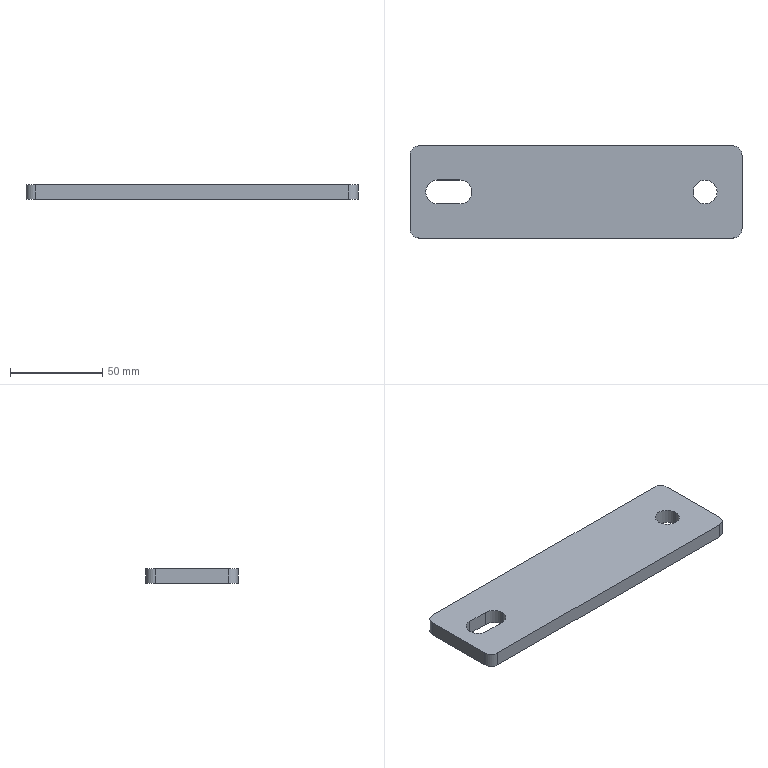Part | STEP file | IN-01-01-03-02 | 1 solid | 17 faces | box 180 x 50 x 8 mm | volume 68457 mm3 | cylinder 9 | plane 8 | commonest cylinder face diameters 13 x5 10 x4
STEP:
#1=CARTESIAN_POINT('',(0.,0.,0.));
#2=DIRECTION('',(0.,0.,1.));
#3=DIRECTION('',(1.,0.,0.));
#4=AXIS2_PLACEMENT_3D('',#1,#2,#3);
#5=CARTESIAN_POINT('',(27.,-18.5,8.));
#6=VERTEX_POINT('',#5);
#7=CARTESIAN_POINT('',(27.,-18.5,0.));
#8=VERTEX_POINT('',#7);
#9=CARTESIAN_POINT('',(27.,-18.5,0.));
#10=DIRECTION('',(0.,0.,-1.));
#11=VECTOR('',#10,1.);
#12=LINE('',#9,#11);
#13=CARTESIAN_POINT('',(27.,-25.,0.));
#14=DIRECTION('',(0.,0.,1.));
#15=DIRECTION('',(1.,0.,0.));
#16=AXIS2_PLACEMENT_3D('',#13,#14,#15);
#17=CYLINDRICAL_SURFACE('',#16,6.5);
#18=CARTESIAN_POINT('',(1.571,0.));
#19=DIRECTION('',(0.,-1.));
#20=VECTOR('',#19,1.);
#21=LINE('',#18,#20);
#22=(GEOMETRIC_REPRESENTATION_CONTEXT(2)PARAMETRIC_REPRESENTATION_CONTEXT()REPRESENTATION_CONTEXT('',''));
#23=DEFINITIONAL_REPRESENTATION('',(#21),#22);
#24=PCURVE('',#17,#23);
#25=CARTESIAN_POINT('',(27.,-18.5,0.));
#26=DIRECTION('',(0.,1.,0.));
#27=DIRECTION('',(0.,0.,1.));
#28=AXIS2_PLACEMENT_3D('',#25,#26,#27);
#29=PLANE('',#28);
#30=CARTESIAN_POINT('',(0.,0.));
#31=DIRECTION('',(-1.,0.));
#32=VECTOR('',#31,1.);
#33=LINE('',#30,#32);
#34=(GEOMETRIC_REPRESENTATION_CONTEXT(2)PARAMETRIC_REPRESENTATION_CONTEXT()REPRESENTATION_CONTEXT('',''));
#35=DEFINITIONAL_REPRESENTATION('',(#33),#34);
#36=PCURVE('',#29,#35);
#37=SURFACE_CURVE('',#12,(#24,#36),.PCURVE_S1.);
#38=EDGE_CURVE('',#6,#8,#37,.T.);
#39=ORIENTED_EDGE('',*,*,#38,.F.);
#40=CARTESIAN_POINT('',(33.5,-25.,8.));
#41=VERTEX_POINT('',#40);
#42=CARTESIAN_POINT('',(27.,-25.,8.));
#43=DIRECTION('',(0.,0.,-1.));
#44=DIRECTION('',(1.,0.,0.));
#45=AXIS2_PLACEMENT_3D('',#42,#43,#44);
#46=CIRCLE('',#45,6.5);
#47=CARTESIAN_POINT('',(6.283,8.));
#48=DIRECTION('',(-1.,0.));
#49=VECTOR('',#48,1.);
#50=LINE('',#47,#49);
#51=(GEOMETRIC_REPRESENTATION_CONTEXT(2)PARAMETRIC_REPRESENTATION_CONTEXT()REPRESENTATION_CONTEXT('',''));
#52=DEFINITIONAL_REPRESENTATION('',(#50),#51);
#53=PCURVE('',#17,#52);
#54=CARTESIAN_POINT('',(90.,-25.,8.));
#55=DIRECTION('',(0.,0.,1.));
#56=DIRECTION('',(1.,0.,0.));
#57=AXIS2_PLACEMENT_3D('',#54,#55,#56);
#58=PLANE('',#57);
#59=CARTESIAN_POINT('',(-56.5,0.));
#60=CARTESIAN_POINT('',(-56.5,-11.258));
#61=CARTESIAN_POINT('',(-66.25,-5.629));
#62=CARTESIAN_POINT('',(-76.,0.));
#63=CARTESIAN_POINT('',(-66.25,5.629));
#64=CARTESIAN_POINT('',(-56.5,11.258));
#65=CARTESIAN_POINT('',(-56.5,0.));
#66=(BOUNDED_CURVE()B_SPLINE_CURVE(2,(#59,#60,#61,#62,#63,#64,#65),.UNSPECIFIED.,.T.,.F.)B_SPLINE_CURVE_WITH_KNOTS((1,2,2,2,2,1),(-2.094,0.,2.094,4.189,6.283,8.378),.UNSPECIFIED.)CURVE()GEOMETRIC_REPRESENTATION_ITEM()RATIONAL_B_SPLINE_CURVE((1.,0.5,1.,0.5,1.,0.5,1.))REPRESENTATION_ITEM(''));
#67=(GEOMETRIC_REPRESENTATION_CONTEXT(2)PARAMETRIC_REPRESENTATION_CONTEXT()REPRESENTATION_CONTEXT('',''));
#68=DEFINITIONAL_REPRESENTATION('',(#66),#67);
#69=PCURVE('',#58,#68);
#70=SURFACE_CURVE('',#46,(#53,#69),.PCURVE_S1.);
#71=EDGE_CURVE('',#6,#41,#70,.T.);
#72=ORIENTED_EDGE('',*,*,#71,.T.);
#73=CARTESIAN_POINT('',(33.5,-25.,0.));
#74=VERTEX_POINT('',#73);
#75=CARTESIAN_POINT('',(33.5,-25.,0.));
#76=DIRECTION('',(0.,0.,1.));
#77=VECTOR('',#76,1.);
#78=LINE('',#75,#77);
#79=CARTESIAN_POINT('',(0.,0.));
#80=DIRECTION('',(0.,1.));
#81=VECTOR('',#80,1.);
#82=LINE('',#79,#81);
#83=(GEOMETRIC_REPRESENTATION_CONTEXT(2)PARAMETRIC_REPRESENTATION_CONTEXT()REPRESENTATION_CONTEXT('',''));
#84=DEFINITIONAL_REPRESENTATION('',(#82),#83);
#85=PCURVE('',#17,#84);
#86=CARTESIAN_POINT('',(27.,-25.,0.));
#87=DIRECTION('',(0.,0.,1.));
#88=DIRECTION('',(1.,0.,0.));
#89=AXIS2_PLACEMENT_3D('',#86,#87,#88);
#90=CYLINDRICAL_SURFACE('',#89,6.5);
#91=CARTESIAN_POINT('',(6.283,0.));
#92=DIRECTION('',(0.,1.));
#93=VECTOR('',#92,1.);
#94=LINE('',#91,#93);
#95=(GEOMETRIC_REPRESENTATION_CONTEXT(2)PARAMETRIC_REPRESENTATION_CONTEXT()REPRESENTATION_CONTEXT('',''));
#96=DEFINITIONAL_REPRESENTATION('',(#94),#95);
#97=PCURVE('',#90,#96);
#98=SURFACE_CURVE('',#78,(#85,#97),.PCURVE_S1.);
#99=EDGE_CURVE('',#74,#41,#98,.T.);
#100=ORIENTED_EDGE('',*,*,#99,.F.);
#101=CARTESIAN_POINT('',(27.,-25.,0.));
#102=DIRECTION('',(0.,0.,-1.));
#103=DIRECTION('',(1.,0.,0.));
#104=AXIS2_PLACEMENT_3D('',#101,#102,#103);
#105=CIRCLE('',#104,6.5);
#106=CARTESIAN_POINT('',(6.283,0.));
#107=DIRECTION('',(-1.,0.));
#108=VECTOR('',#107,1.);
#109=LINE('',#106,#108);
#110=(GEOMETRIC_REPRESENTATION_CONTEXT(2)PARAMETRIC_REPRESENTATION_CONTEXT()REPRESENTATION_CONTEXT('',''));
#111=DEFINITIONAL_REPRESENTATION('',(#109),#110);
#112=PCURVE('',#17,#111);
#113=CARTESIAN_POINT('',(90.,-25.,0.));
#114=DIRECTION('',(0.,0.,1.));
#115=DIRECTION('',(1.,0.,0.));
#116=AXIS2_PLACEMENT_3D('',#113,#114,#115);
#117=PLANE('',#116);
#118=CARTESIAN_POINT('',(-56.5,0.));
#119=CARTESIAN_POINT('',(-56.5,-11.258));
#120=CARTESIAN_POINT('',(-66.25,-5.629));
#121=CARTESIAN_POINT('',(-76.,0.));
#122=CARTESIAN_POINT('',(-66.25,5.629));
#123=CARTESIAN_POINT('',(-56.5,11.258));
#124=CARTESIAN_POINT('',(-56.5,0.));
#125=(BOUNDED_CURVE()B_SPLINE_CURVE(2,(#118,#119,#120,#121,#122,#123,#124),.UNSPECIFIED.,.T.,.F.)B_SPLINE_CURVE_WITH_KNOTS((1,2,2,2,2,1),(-2.094,0.,2.094,4.189,6.283,8.378),.UNSPECIFIED.)CURVE()GEOMETRIC_REPRESENTATION_ITEM()RATIONAL_B_SPLINE_CURVE((1.,0.5,1.,0.5,1.,0.5,1.))REPRESENTATION_ITEM(''));
#126=(GEOMETRIC_REPRESENTATION_CONTEXT(2)PARAMETRIC_REPRESENTATION_CONTEXT()REPRESENTATION_CONTEXT('',''));
#127=DEFINITIONAL_REPRESENTATION('',(#125),#126);
#128=PCURVE('',#117,#127);
#129=SURFACE_CURVE('',#105,(#112,#128),.PCURVE_S1.);
#130=EDGE_CURVE('',#8,#74,#129,.T.);
#131=ORIENTED_EDGE('',*,*,#130,.F.);
#132=EDGE_LOOP('',(#39,#72,#100,#131));
#133=FACE_BOUND('',#132,.F.);
#134=ADVANCED_FACE('',(#133),#17,.F.);
#135=CARTESIAN_POINT('',(166.5,-25.,0.));
#136=VERTEX_POINT('',#135);
#137=CARTESIAN_POINT('',(166.5,-25.,8.));
#138=VERTEX_POINT('',#137);
#139=CARTESIAN_POINT('',(166.5,-25.,0.));
#140=DIRECTION('',(0.,0.,1.));
#141=VECTOR('',#140,1.);
#142=LINE('',#139,#141);
#143=CARTESIAN_POINT('',(160.,-25.,0.));
#144=DIRECTION('',(0.,0.,1.));
#145=DIRECTION('',(1.,0.,0.));
#146=AXIS2_PLACEMENT_3D('',#143,#144,#145);
#147=CYLINDRICAL_SURFACE('',#146,6.5);
#148=CARTESIAN_POINT('',(6.283,0.));
#149=DIRECTION('',(0.,1.));
#150=VECTOR('',#149,1.);
#151=LINE('',#148,#150);
#152=(GEOMETRIC_REPRESENTATION_CONTEXT(2)PARAMETRIC_REPRESENTATION_CONTEXT()REPRESENTATION_CONTEXT('',''));
#153=DEFINITIONAL_REPRESENTATION('',(#151),#152);
#154=PCURVE('',#147,#153);
#155=CARTESIAN_POINT('',(160.,-25.,0.));
#156=DIRECTION('',(0.,0.,1.));
#157=DIRECTION('',(1.,0.,0.));
#158=AXIS2_PLACEMENT_3D('',#155,#156,#157);
#159=CYLINDRICAL_SURFACE('',#158,6.5);
#160=CARTESIAN_POINT('',(0.,0.));
#161=DIRECTION('',(0.,1.));
#162=VECTOR('',#161,1.);
#163=LINE('',#160,#162);
#164=(GEOMETRIC_REPRESENTATION_CONTEXT(2)PARAMETRIC_REPRESENTATION_CONTEXT()REPRESENTATION_CONTEXT('',''));
#165=DEFINITIONAL_REPRESENTATION('',(#163),#164);
#166=PCURVE('',#159,#165);
#167=SURFACE_CURVE('',#142,(#154,#166),.PCURVE_S1.);
#168=EDGE_CURVE('',#136,#138,#167,.T.);
#169=ORIENTED_EDGE('',*,*,#168,.T.);
#170=CARTESIAN_POINT('',(153.5,-25.,8.));
#171=VERTEX_POINT('',#170);
#172=CARTESIAN_POINT('',(160.,-25.,8.));
#173=DIRECTION('',(0.,0.,-1.));
#174=DIRECTION('',(1.,0.,0.));
#175=AXIS2_PLACEMENT_3D('',#172,#173,#174);
#176=CIRCLE('',#175,6.5);
#177=CARTESIAN_POINT('',(6.283,8.));
#178=DIRECTION('',(-1.,0.));
#179=VECTOR('',#178,1.);
#180=LINE('',#177,#179);
#181=(GEOMETRIC_REPRESENTATION_CONTEXT(2)PARAMETRIC_REPRESENTATION_CONTEXT()REPRESENTATION_CONTEXT('',''));
#182=DEFINITIONAL_REPRESENTATION('',(#180),#181);
#183=PCURVE('',#147,#182);
#184=CARTESIAN_POINT('',(76.5,0.));
#185=CARTESIAN_POINT('',(76.5,-11.258));
#186=CARTESIAN_POINT('',(66.75,-5.629));
#187=CARTESIAN_POINT('',(57.,0.));
#188=CARTESIAN_POINT('',(66.75,5.629));
#189=CARTESIAN_POINT('',(76.5,11.258));
#190=CARTESIAN_POINT('',(76.5,0.));
#191=(BOUNDED_CURVE()B_SPLINE_CURVE(2,(#184,#185,#186,#187,#188,#189,#190),.UNSPECIFIED.,.T.,.F.)B_SPLINE_CURVE_WITH_KNOTS((1,2,2,2,2,1),(-2.094,0.,2.094,4.189,6.283,8.378),.UNSPECIFIED.)CURVE()GEOMETRIC_REPRESENTATION_ITEM()RATIONAL_B_SPLINE_CURVE((1.,0.5,1.,0.5,1.,0.5,1.))REPRESENTATION_ITEM(''));
#192=(GEOMETRIC_REPRESENTATION_CONTEXT(2)PARAMETRIC_REPRESENTATION_CONTEXT()REPRESENTATION_CONTEXT('',''));
#193=DEFINITIONAL_REPRESENTATION('',(#191),#192);
#194=PCURVE('',#58,#193);
#195=SURFACE_CURVE('',#176,(#183,#194),.PCURVE_S1.);
#196=EDGE_CURVE('',#138,#171,#195,.T.);
#197=ORIENTED_EDGE('',*,*,#196,.T.);
#198=CARTESIAN_POINT('',(153.5,-25.,0.));
#199=VERTEX_POINT('',#198);
#200=CARTESIAN_POINT('',(153.5,-25.,0.));
#201=DIRECTION('',(0.,0.,1.));
#202=VECTOR('',#201,1.);
#203=LINE('',#200,#202);
#204=CARTESIAN_POINT('',(3.142,0.));
#205=DIRECTION('',(0.,1.));
#206=VECTOR('',#205,1.);
#207=LINE('',#204,#206);
#208=(GEOMETRIC_REPRESENTATION_CONTEXT(2)PARAMETRIC_REPRESENTATION_CONTEXT()REPRESENTATION_CONTEXT('',''));
#209=DEFINITIONAL_REPRESENTATION('',(#207),#208);
#210=PCURVE('',#147,#209);
#211=CARTESIAN_POINT('',(3.142,0.));
#212=DIRECTION('',(0.,1.));
#213=VECTOR('',#212,1.);
#214=LINE('',#211,#213);
#215=(GEOMETRIC_REPRESENTATION_CONTEXT(2)PARAMETRIC_REPRESENTATION_CONTEXT()REPRESENTATION_CONTEXT('',''));
#216=DEFINITIONAL_REPRESENTATION('',(#214),#215);
#217=PCURVE('',#159,#216);
#218=SURFACE_CURVE('',#203,(#210,#217),.PCURVE_S1.);
#219=EDGE_CURVE('',#199,#171,#218,.T.);
#220=ORIENTED_EDGE('',*,*,#219,.F.);
#221=CARTESIAN_POINT('',(160.,-25.,0.));
#222=DIRECTION('',(0.,0.,-1.));
#223=DIRECTION('',(1.,0.,0.));
#224=AXIS2_PLACEMENT_3D('',#221,#222,#223);
#225=CIRCLE('',#224,6.5);
#226=CARTESIAN_POINT('',(6.283,0.));
#227=DIRECTION('',(-1.,0.));
#228=VECTOR('',#227,1.);
#229=LINE('',#226,#228);
#230=(GEOMETRIC_REPRESENTATION_CONTEXT(2)PARAMETRIC_REPRESENTATION_CONTEXT()REPRESENTATION_CONTEXT('',''));
#231=DEFINITIONAL_REPRESENTATION('',(#229),#230);
#232=PCURVE('',#147,#231);
#233=CARTESIAN_POINT('',(76.5,0.));
#234=CARTESIAN_POINT('',(76.5,-11.258));
#235=CARTESIAN_POINT('',(66.75,-5.629));
#236=CARTESIAN_POINT('',(57.,0.));
#237=CARTESIAN_POINT('',(66.75,5.629));
#238=CARTESIAN_POINT('',(76.5,11.258));
#239=CARTESIAN_POINT('',(76.5,0.));
#240=(BOUNDED_CURVE()B_SPLINE_CURVE(2,(#233,#234,#235,#236,#237,#238,#239),.UNSPECIFIED.,.T.,.F.)B_SPLINE_CURVE_WITH_KNOTS((1,2,2,2,2,1),(-2.094,0.,2.094,4.189,6.283,8.378),.UNSPECIFIED.)CURVE()GEOMETRIC_REPRESENTATION_ITEM()RATIONAL_B_SPLINE_CURVE((1.,0.5,1.,0.5,1.,0.5,1.))REPRESENTATION_ITEM(''));
#241=(GEOMETRIC_REPRESENTATION_CONTEXT(2)PARAMETRIC_REPRESENTATION_CONTEXT()REPRESENTATION_CONTEXT('',''));
#242=DEFINITIONAL_REPRESENTATION('',(#240),#241);
#243=PCURVE('',#117,#242);
#244=SURFACE_CURVE('',#225,(#232,#243),.PCURVE_S1.);
#245=EDGE_CURVE('',#136,#199,#244,.T.);
#246=ORIENTED_EDGE('',*,*,#245,.F.);
#247=EDGE_LOOP('',(#169,#197,#220,#246));
#248=FACE_BOUND('',#247,.F.);
#249=ADVANCED_FACE('',(#248),#147,.F.);
#250=CARTESIAN_POINT('',(15.,-31.5,0.));
#251=VERTEX_POINT('',#250);
#252=CARTESIAN_POINT('',(15.,-18.5,0.));
#253=VERTEX_POINT('',#252);
#254=CARTESIAN_POINT('',(15.,-25.,0.));
#255=DIRECTION('',(0.,0.,-1.));
#256=DIRECTION('',(1.,0.,0.));
#257=AXIS2_PLACEMENT_3D('',#254,#255,#256);
#258=CIRCLE('',#257,6.5);
#259=CARTESIAN_POINT('',(-68.5,0.));
#260=CARTESIAN_POINT('',(-68.5,-11.258));
#261=CARTESIAN_POINT('',(-78.25,-5.629));
#262=CARTESIAN_POINT('',(-88.,0.));
#263=CARTESIAN_POINT('',(-78.25,5.629));
#264=CARTESIAN_POINT('',(-68.5,11.258));
#265=CARTESIAN_POINT('',(-68.5,0.));
#266=(BOUNDED_CURVE()B_SPLINE_CURVE(2,(#259,#260,#261,#262,#263,#264,#265),.UNSPECIFIED.,.T.,.F.)B_SPLINE_CURVE_WITH_KNOTS((1,2,2,2,2,1),(-2.094,0.,2.094,4.189,6.283,8.378),.UNSPECIFIED.)CURVE()GEOMETRIC_REPRESENTATION_ITEM()RATIONAL_B_SPLINE_CURVE((1.,0.5,1.,0.5,1.,0.5,1.))REPRESENTATION_ITEM(''));
#267=(GEOMETRIC_REPRESENTATION_CONTEXT(2)PARAMETRIC_REPRESENTATION_CONTEXT()REPRESENTATION_CONTEXT('',''));
#268=DEFINITIONAL_REPRESENTATION('',(#266),#267);
#269=PCURVE('',#117,#268);
#270=CARTESIAN_POINT('',(15.,-25.,0.));
#271=DIRECTION('',(0.,0.,1.));
#272=DIRECTION('',(1.,0.,0.));
#273=AXIS2_PLACEMENT_3D('',#270,#271,#272);
#274=CYLINDRICAL_SURFACE('',#273,6.5);
#275=CARTESIAN_POINT('',(6.283,0.));
#276=DIRECTION('',(-1.,0.));
#277=VECTOR('',#276,1.);
#278=LINE('',#275,#277);
#279=(GEOMETRIC_REPRESENTATION_CONTEXT(2)PARAMETRIC_REPRESENTATION_CONTEXT()REPRESENTATION_CONTEXT('',''));
#280=DEFINITIONAL_REPRESENTATION('',(#278),#279);
#281=PCURVE('',#274,#280);
#282=SURFACE_CURVE('',#258,(#269,#281),.PCURVE_S1.);
#283=EDGE_CURVE('',#251,#253,#282,.T.);
#284=ORIENTED_EDGE('',*,*,#283,.F.);
#285=CARTESIAN_POINT('',(27.,-31.5,0.));
#286=VERTEX_POINT('',#285);
#287=CARTESIAN_POINT('',(90.,-31.5,0.));
#288=DIRECTION('',(-1.,0.,0.));
#289=VECTOR('',#288,1.);
#290=LINE('',#287,#289);
#291=CARTESIAN_POINT('',(0.,-6.5));
#292=DIRECTION('',(-1.,0.));
#293=VECTOR('',#292,1.);
#294=LINE('',#291,#293);
#295=(GEOMETRIC_REPRESENTATION_CONTEXT(2)PARAMETRIC_REPRESENTATION_CONTEXT()REPRESENTATION_CONTEXT('',''));
#296=DEFINITIONAL_REPRESENTATION('',(#294),#295);
#297=PCURVE('',#117,#296);
#298=CARTESIAN_POINT('',(15.,-31.5,0.));
#299=DIRECTION('',(0.,-1.,0.));
#300=DIRECTION('',(0.,0.,-1.));
#301=AXIS2_PLACEMENT_3D('',#298,#299,#300);
#302=PLANE('',#301);
#303=CARTESIAN_POINT('',(0.,75.));
#304=DIRECTION('',(0.,-1.));
#305=VECTOR('',#304,1.);
#306=LINE('',#303,#305);
#307=(GEOMETRIC_REPRESENTATION_CONTEXT(2)PARAMETRIC_REPRESENTATION_CONTEXT()REPRESENTATION_CONTEXT('',''));
#308=DEFINITIONAL_REPRESENTATION('',(#306),#307);
#309=PCURVE('',#302,#308);
#310=SURFACE_CURVE('',#290,(#297,#309),.PCURVE_S1.);
#311=EDGE_CURVE('',#286,#251,#310,.T.);
#312=ORIENTED_EDGE('',*,*,#311,.F.);
#313=CARTESIAN_POINT('',(27.,-25.,0.));
#314=DIRECTION('',(0.,0.,-1.));
#315=DIRECTION('',(1.,0.,0.));
#316=AXIS2_PLACEMENT_3D('',#313,#314,#315);
#317=CIRCLE('',#316,6.5);
#318=CARTESIAN_POINT('',(-56.5,0.));
#319=CARTESIAN_POINT('',(-56.5,-11.258));
#320=CARTESIAN_POINT('',(-66.25,-5.629));
#321=CARTESIAN_POINT('',(-76.,0.));
#322=CARTESIAN_POINT('',(-66.25,5.629));
#323=CARTESIAN_POINT('',(-56.5,11.258));
#324=CARTESIAN_POINT('',(-56.5,0.));
#325=(BOUNDED_CURVE()B_SPLINE_CURVE(2,(#318,#319,#320,#321,#322,#323,#324),.UNSPECIFIED.,.T.,.F.)B_SPLINE_CURVE_WITH_KNOTS((1,2,2,2,2,1),(-2.094,0.,2.094,4.189,6.283,8.378),.UNSPECIFIED.)CURVE()GEOMETRIC_REPRESENTATION_ITEM()RATIONAL_B_SPLINE_CURVE((1.,0.5,1.,0.5,1.,0.5,1.))REPRESENTATION_ITEM(''));
#326=(GEOMETRIC_REPRESENTATION_CONTEXT(2)PARAMETRIC_REPRESENTATION_CONTEXT()REPRESENTATION_CONTEXT('',''));
#327=DEFINITIONAL_REPRESENTATION('',(#325),#326);
#328=PCURVE('',#117,#327);
#329=CARTESIAN_POINT('',(6.283,0.));
#330=DIRECTION('',(-1.,0.));
#331=VECTOR('',#330,1.);
#332=LINE('',#329,#331);
#333=(GEOMETRIC_REPRESENTATION_CONTEXT(2)PARAMETRIC_REPRESENTATION_CONTEXT()REPRESENTATION_CONTEXT('',''));
#334=DEFINITIONAL_REPRESENTATION('',(#332),#333);
#335=PCURVE('',#90,#334);
#336=SURFACE_CURVE('',#317,(#328,#335),.PCURVE_S1.);
#337=EDGE_CURVE('',#74,#286,#336,.T.);
#338=ORIENTED_EDGE('',*,*,#337,.F.);
#339=ORIENTED_EDGE('',*,*,#130,.F.);
#340=CARTESIAN_POINT('',(90.,-18.5,0.));
#341=DIRECTION('',(1.,0.,0.));
#342=VECTOR('',#341,1.);
#343=LINE('',#340,#342);
#344=CARTESIAN_POINT('',(0.,6.5));
#345=DIRECTION('',(1.,0.));
#346=VECTOR('',#345,1.);
#347=LINE('',#344,#346);
#348=(GEOMETRIC_REPRESENTATION_CONTEXT(2)PARAMETRIC_REPRESENTATION_CONTEXT()REPRESENTATION_CONTEXT('',''));
#349=DEFINITIONAL_REPRESENTATION('',(#347),#348);
#350=PCURVE('',#117,#349);
#351=CARTESIAN_POINT('',(0.,63.));
#352=DIRECTION('',(0.,1.));
#353=VECTOR('',#352,1.);
#354=LINE('',#351,#353);
#355=(GEOMETRIC_REPRESENTATION_CONTEXT(2)PARAMETRIC_REPRESENTATION_CONTEXT()REPRESENTATION_CONTEXT('',''));
#356=DEFINITIONAL_REPRESENTATION('',(#354),#355);
#357=PCURVE('',#29,#356);
#358=SURFACE_CURVE('',#343,(#350,#357),.PCURVE_S1.);
#359=EDGE_CURVE('',#253,#8,#358,.T.);
#360=ORIENTED_EDGE('',*,*,#359,.F.);
#361=EDGE_LOOP('',(#284,#312,#338,#339,#360));
#362=FACE_BOUND('',#361,.T.);
#363=ORIENTED_EDGE('',*,*,#245,.F.);
#364=CARTESIAN_POINT('',(160.,-25.,0.));
#365=DIRECTION('',(0.,0.,-1.));
#366=DIRECTION('',(1.,0.,0.));
#367=AXIS2_PLACEMENT_3D('',#364,#365,#366);
#368=CIRCLE('',#367,6.5);
#369=CARTESIAN_POINT('',(76.5,0.));
#370=CARTESIAN_POINT('',(76.5,-11.258));
#371=CARTESIAN_POINT('',(66.75,-5.629));
#372=CARTESIAN_POINT('',(57.,0.));
#373=CARTESIAN_POINT('',(66.75,5.629));
#374=CARTESIAN_POINT('',(76.5,11.258));
#375=CARTESIAN_POINT('',(76.5,0.));
#376=(BOUNDED_CURVE()B_SPLINE_CURVE(2,(#369,#370,#371,#372,#373,#374,#375),.UNSPECIFIED.,.T.,.F.)B_SPLINE_CURVE_WITH_KNOTS((1,2,2,2,2,1),(-2.094,0.,2.094,4.189,6.283,8.378),.UNSPECIFIED.)CURVE()GEOMETRIC_REPRESENTATION_ITEM()RATIONAL_B_SPLINE_CURVE((1.,0.5,1.,0.5,1.,0.5,1.))REPRESENTATION_ITEM(''));
#377=(GEOMETRIC_REPRESENTATION_CONTEXT(2)PARAMETRIC_REPRESENTATION_CONTEXT()REPRESENTATION_CONTEXT('',''));
#378=DEFINITIONAL_REPRESENTATION('',(#376),#377);
#379=PCURVE('',#117,#378);
#380=CARTESIAN_POINT('',(6.283,0.));
#381=DIRECTION('',(-1.,0.));
#382=VECTOR('',#381,1.);
#383=LINE('',#380,#382);
#384=(GEOMETRIC_REPRESENTATION_CONTEXT(2)PARAMETRIC_REPRESENTATION_CONTEXT()REPRESENTATION_CONTEXT('',''));
#385=DEFINITIONAL_REPRESENTATION('',(#383),#384);
#386=PCURVE('',#159,#385);
#387=SURFACE_CURVE('',#368,(#379,#386),.PCURVE_S1.);
#388=EDGE_CURVE('',#199,#136,#387,.T.);
#389=ORIENTED_EDGE('',*,*,#388,.F.);
#390=EDGE_LOOP('',(#363,#389));
#391=FACE_BOUND('',#390,.T.);
#392=CARTESIAN_POINT('',(5.,0.,0.));
#393=VERTEX_POINT('',#392);
#394=CARTESIAN_POINT('',(0.,-5.,0.));
#395=VERTEX_POINT('',#394);
#396=CARTESIAN_POINT('',(5.,-5.,0.));
#397=DIRECTION('',(0.,0.,1.));
#398=DIRECTION('',(1.,0.,0.));
#399=AXIS2_PLACEMENT_3D('',#396,#397,#398);
#400=CIRCLE('',#399,5.);
#401=CARTESIAN_POINT('',(-85.,20.));
#402=DIRECTION('',(1.,0.));
#403=AXIS2_PLACEMENT_2D('',#401,#402);
#404=CIRCLE('',#403,5.);
#405=(GEOMETRIC_REPRESENTATION_CONTEXT(2)PARAMETRIC_REPRESENTATION_CONTEXT()REPRESENTATION_CONTEXT('',''));
#406=DEFINITIONAL_REPRESENTATION('',(#404),#405);
#407=PCURVE('',#117,#406);
#408=CARTESIAN_POINT('',(5.,-5.,0.));
#409=DIRECTION('',(0.,0.,1.));
#410=DIRECTION('',(1.,0.,0.));
#411=AXIS2_PLACEMENT_3D('',#408,#409,#410);
#412=CYLINDRICAL_SURFACE('',#411,5.);
#413=CARTESIAN_POINT('',(0.,0.));
#414=DIRECTION('',(1.,0.));
#415=VECTOR('',#414,1.);
#416=LINE('',#413,#415);
#417=(GEOMETRIC_REPRESENTATION_CONTEXT(2)PARAMETRIC_REPRESENTATION_CONTEXT()REPRESENTATION_CONTEXT('',''));
#418=DEFINITIONAL_REPRESENTATION('',(#416),#417);
#419=PCURVE('',#412,#418);
#420=SURFACE_CURVE('',#400,(#407,#419),.PCURVE_S1.);
#421=EDGE_CURVE('',#393,#395,#420,.T.);
#422=ORIENTED_EDGE('',*,*,#421,.F.);
#423=CARTESIAN_POINT('',(175.,0.,0.));
#424=VERTEX_POINT('',#423);
#425=CARTESIAN_POINT('',(90.,0.,0.));
#426=DIRECTION('',(-1.,0.,0.));
#427=VECTOR('',#426,1.);
#428=LINE('',#425,#427);
#429=CARTESIAN_POINT('',(0.,25.));
#430=DIRECTION('',(-1.,0.));
#431=VECTOR('',#430,1.);
#432=LINE('',#429,#431);
#433=(GEOMETRIC_REPRESENTATION_CONTEXT(2)PARAMETRIC_REPRESENTATION_CONTEXT()REPRESENTATION_CONTEXT('',''));
#434=DEFINITIONAL_REPRESENTATION('',(#432),#433);
#435=PCURVE('',#117,#434);
#436=CARTESIAN_POINT('',(175.,0.,0.));
#437=DIRECTION('',(0.,1.,0.));
#438=DIRECTION('',(-1.,0.,0.));
#439=AXIS2_PLACEMENT_3D('',#436,#437,#438);
#440=PLANE('',#439);
#441=CARTESIAN_POINT('',(85.,0.));
#442=DIRECTION('',(1.,0.));
#443=VECTOR('',#442,1.);
#444=LINE('',#441,#443);
#445=(GEOMETRIC_REPRESENTATION_CONTEXT(2)PARAMETRIC_REPRESENTATION_CONTEXT()REPRESENTATION_CONTEXT('',''));
#446=DEFINITIONAL_REPRESENTATION('',(#444),#445);
#447=PCURVE('',#440,#446);
#448=SURFACE_CURVE('',#428,(#435,#447),.PCURVE_S1.);
#449=EDGE_CURVE('',#424,#393,#448,.T.);
#450=ORIENTED_EDGE('',*,*,#449,.F.);
#451=CARTESIAN_POINT('',(180.,-5.,0.));
#452=VERTEX_POINT('',#451);
#453=CARTESIAN_POINT('',(175.,-5.,0.));
#454=DIRECTION('',(0.,0.,1.));
#455=DIRECTION('',(1.,0.,0.));
#456=AXIS2_PLACEMENT_3D('',#453,#454,#455);
#457=CIRCLE('',#456,5.);
#458=CARTESIAN_POINT('',(85.,20.));
#459=DIRECTION('',(1.,0.));
#460=AXIS2_PLACEMENT_2D('',#458,#459);
#461=CIRCLE('',#460,5.);
#462=(GEOMETRIC_REPRESENTATION_CONTEXT(2)PARAMETRIC_REPRESENTATION_CONTEXT()REPRESENTATION_CONTEXT('',''));
#463=DEFINITIONAL_REPRESENTATION('',(#461),#462);
#464=PCURVE('',#117,#463);
#465=CARTESIAN_POINT('',(175.,-5.,0.));
#466=DIRECTION('',(0.,0.,1.));
#467=DIRECTION('',(1.,0.,0.));
#468=AXIS2_PLACEMENT_3D('',#465,#466,#467);
#469=CYLINDRICAL_SURFACE('',#468,5.);
#470=CARTESIAN_POINT('',(0.,0.));
#471=DIRECTION('',(1.,0.));
#472=VECTOR('',#471,1.);
#473=LINE('',#470,#472);
#474=(GEOMETRIC_REPRESENTATION_CONTEXT(2)PARAMETRIC_REPRESENTATION_CONTEXT()REPRESENTATION_CONTEXT('',''));
#475=DEFINITIONAL_REPRESENTATION('',(#473),#474);
#476=PCURVE('',#469,#475);
#477=SURFACE_CURVE('',#457,(#464,#476),.PCURVE_S1.);
#478=EDGE_CURVE('',#452,#424,#477,.T.);
#479=ORIENTED_EDGE('',*,*,#478,.F.);
#480=CARTESIAN_POINT('',(180.,-45.,0.));
#481=VERTEX_POINT('',#480);
#482=CARTESIAN_POINT('',(180.,-25.,0.));
#483=DIRECTION('',(0.,1.,0.));
#484=VECTOR('',#483,1.);
#485=LINE('',#482,#484);
#486=CARTESIAN_POINT('',(90.,0.));
#487=DIRECTION('',(0.,1.));
#488=VECTOR('',#487,1.);
#489=LINE('',#486,#488);
#490=(GEOMETRIC_REPRESENTATION_CONTEXT(2)PARAMETRIC_REPRESENTATION_CONTEXT()REPRESENTATION_CONTEXT('',''));
#491=DEFINITIONAL_REPRESENTATION('',(#489),#490);
#492=PCURVE('',#117,#491);
#493=CARTESIAN_POINT('',(180.,-45.,0.));
#494=DIRECTION('',(1.,0.,0.));
#495=DIRECTION('',(0.,0.,-1.));
#496=AXIS2_PLACEMENT_3D('',#493,#494,#495);
#497=PLANE('',#496);
#498=CARTESIAN_POINT('',(0.,20.));
#499=DIRECTION('',(0.,1.));
#500=VECTOR('',#499,1.);
#501=LINE('',#498,#500);
#502=(GEOMETRIC_REPRESENTATION_CONTEXT(2)PARAMETRIC_REPRESENTATION_CONTEXT()REPRESENTATION_CONTEXT('',''));
#503=DEFINITIONAL_REPRESENTATION('',(#501),#502);
#504=PCURVE('',#497,#503);
#505=SURFACE_CURVE('',#485,(#492,#504),.PCURVE_S1.);
#506=EDGE_CURVE('',#481,#452,#505,.T.);
#507=ORIENTED_EDGE('',*,*,#506,.F.);
#508=CARTESIAN_POINT('',(175.,-50.,0.));
#509=VERTEX_POINT('',#508);
#510=CARTESIAN_POINT('',(175.,-45.,0.));
#511=DIRECTION('',(0.,0.,1.));
#512=DIRECTION('',(1.,0.,0.));
#513=AXIS2_PLACEMENT_3D('',#510,#511,#512);
#514=CIRCLE('',#513,5.);
#515=CARTESIAN_POINT('',(85.,-20.));
#516=DIRECTION('',(1.,0.));
#517=AXIS2_PLACEMENT_2D('',#515,#516);
#518=CIRCLE('',#517,5.);
#519=(GEOMETRIC_REPRESENTATION_CONTEXT(2)PARAMETRIC_REPRESENTATION_CONTEXT()REPRESENTATION_CONTEXT('',''));
#520=DEFINITIONAL_REPRESENTATION('',(#518),#519);
#521=PCURVE('',#117,#520);
#522=CARTESIAN_POINT('',(175.,-45.,0.));
#523=DIRECTION('',(0.,0.,1.));
#524=DIRECTION('',(1.,0.,0.));
#525=AXIS2_PLACEMENT_3D('',#522,#523,#524);
#526=CYLINDRICAL_SURFACE('',#525,5.);
#527=CARTESIAN_POINT('',(0.,0.));
#528=DIRECTION('',(1.,0.));
#529=VECTOR('',#528,1.);
#530=LINE('',#527,#529);
#531=(GEOMETRIC_REPRESENTATION_CONTEXT(2)PARAMETRIC_REPRESENTATION_CONTEXT()REPRESENTATION_CONTEXT('',''));
#532=DEFINITIONAL_REPRESENTATION('',(#530),#531);
#533=PCURVE('',#526,#532);
#534=SURFACE_CURVE('',#514,(#521,#533),.PCURVE_S1.);
#535=EDGE_CURVE('',#509,#481,#534,.T.);
#536=ORIENTED_EDGE('',*,*,#535,.F.);
#537=CARTESIAN_POINT('',(5.,-50.,0.));
#538=VERTEX_POINT('',#537);
#539=CARTESIAN_POINT('',(90.,-50.,0.));
#540=DIRECTION('',(1.,0.,0.));
#541=VECTOR('',#540,1.);
#542=LINE('',#539,#541);
#543=CARTESIAN_POINT('',(0.,-25.));
#544=DIRECTION('',(1.,0.));
#545=VECTOR('',#544,1.);
#546=LINE('',#543,#545);
#547=(GEOMETRIC_REPRESENTATION_CONTEXT(2)PARAMETRIC_REPRESENTATION_CONTEXT()REPRESENTATION_CONTEXT('',''));
#548=DEFINITIONAL_REPRESENTATION('',(#546),#547);
#549=PCURVE('',#117,#548);
#550=CARTESIAN_POINT('',(5.,-50.,0.));
#551=DIRECTION('',(0.,-1.,0.));
#552=DIRECTION('',(1.,0.,0.));
#553=AXIS2_PLACEMENT_3D('',#550,#551,#552);
#554=PLANE('',#553);
#555=CARTESIAN_POINT('',(85.,0.));
#556=DIRECTION('',(1.,0.));
#557=VECTOR('',#556,1.);
#558=LINE('',#555,#557);
#559=(GEOMETRIC_REPRESENTATION_CONTEXT(2)PARAMETRIC_REPRESENTATION_CONTEXT()REPRESENTATION_CONTEXT('',''));
#560=DEFINITIONAL_REPRESENTATION('',(#558),#559);
#561=PCURVE('',#554,#560);
#562=SURFACE_CURVE('',#542,(#549,#561),.PCURVE_S1.);
#563=EDGE_CURVE('',#538,#509,#562,.T.);
#564=ORIENTED_EDGE('',*,*,#563,.F.);
#565=CARTESIAN_POINT('',(0.,-45.,0.));
#566=VERTEX_POINT('',#565);
#567=CARTESIAN_POINT('',(5.,-45.,0.));
#568=DIRECTION('',(0.,0.,1.));
#569=DIRECTION('',(1.,0.,0.));
#570=AXIS2_PLACEMENT_3D('',#567,#568,#569);
#571=CIRCLE('',#570,5.);
#572=CARTESIAN_POINT('',(-85.,-20.));
#573=DIRECTION('',(1.,0.));
#574=AXIS2_PLACEMENT_2D('',#572,#573);
#575=CIRCLE('',#574,5.);
#576=(GEOMETRIC_REPRESENTATION_CONTEXT(2)PARAMETRIC_REPRESENTATION_CONTEXT()REPRESENTATION_CONTEXT('',''));
#577=DEFINITIONAL_REPRESENTATION('',(#575),#576);
#578=PCURVE('',#117,#577);
#579=CARTESIAN_POINT('',(5.,-45.,0.));
#580=DIRECTION('',(0.,0.,1.));
#581=DIRECTION('',(1.,0.,0.));
#582=AXIS2_PLACEMENT_3D('',#579,#580,#581);
#583=CYLINDRICAL_SURFACE('',#582,5.);
#584=CARTESIAN_POINT('',(0.,0.));
#585=DIRECTION('',(1.,0.));
#586=VECTOR('',#585,1.);
#587=LINE('',#584,#586);
#588=(GEOMETRIC_REPRESENTATION_CONTEXT(2)PARAMETRIC_REPRESENTATION_CONTEXT()REPRESENTATION_CONTEXT('',''));
#589=DEFINITIONAL_REPRESENTATION('',(#587),#588);
#590=PCURVE('',#583,#589);
#591=SURFACE_CURVE('',#571,(#578,#590),.PCURVE_S1.);
#592=EDGE_CURVE('',#566,#538,#591,.T.);
#593=ORIENTED_EDGE('',*,*,#592,.F.);
#594=CARTESIAN_POINT('',(0.,-25.,0.));
#595=DIRECTION('',(0.,-1.,0.));
#596=VECTOR('',#595,1.);
#597=LINE('',#594,#596);
#598=CARTESIAN_POINT('',(-90.,0.));
#599=DIRECTION('',(0.,-1.));
#600=VECTOR('',#599,1.);
#601=LINE('',#598,#600);
#602=(GEOMETRIC_REPRESENTATION_CONTEXT(2)PARAMETRIC_REPRESENTATION_CONTEXT()REPRESENTATION_CONTEXT('',''));
#603=DEFINITIONAL_REPRESENTATION('',(#601),#602);
#604=PCURVE('',#117,#603);
#605=CARTESIAN_POINT('',(0.,-5.,0.));
#606=DIRECTION('',(-1.,0.,0.));
#607=DIRECTION('',(0.,-1.,0.));
#608=AXIS2_PLACEMENT_3D('',#605,#606,#607);
#609=PLANE('',#608);
#610=CARTESIAN_POINT('',(20.,0.));
#611=DIRECTION('',(1.,0.));
#612=VECTOR('',#611,1.);
#613=LINE('',#610,#612);
#614=(GEOMETRIC_REPRESENTATION_CONTEXT(2)PARAMETRIC_REPRESENTATION_CONTEXT()REPRESENTATION_CONTEXT('',''));
#615=DEFINITIONAL_REPRESENTATION('',(#613),#614);
#616=PCURVE('',#609,#615);
#617=SURFACE_CURVE('',#597,(#604,#616),.PCURVE_S1.);
#618=EDGE_CURVE('',#395,#566,#617,.T.);
#619=ORIENTED_EDGE('',*,*,#618,.F.);
#620=EDGE_LOOP('',(#422,#450,#479,#507,#536,#564,#593,#619));
#621=FACE_BOUND('',#620,.T.);
#622=ADVANCED_FACE('',(#362,#391,#621),#117,.F.);
#623=ORIENTED_EDGE('',*,*,#38,.F.);
#624=CARTESIAN_POINT('',(15.,-18.5,8.));
#625=VERTEX_POINT('',#624);
#626=CARTESIAN_POINT('',(27.,-18.5,8.));
#627=DIRECTION('',(1.,0.,0.));
#628=VECTOR('',#627,1.);
#629=LINE('',#626,#628);
#630=CARTESIAN_POINT('',(8.,0.));
#631=DIRECTION('',(0.,1.));
#632=VECTOR('',#631,1.);
#633=LINE('',#630,#632);
#634=(GEOMETRIC_REPRESENTATION_CONTEXT(2)PARAMETRIC_REPRESENTATION_CONTEXT()REPRESENTATION_CONTEXT('',''));
#635=DEFINITIONAL_REPRESENTATION('',(#633),#634);
#636=PCURVE('',#29,#635);
#637=CARTESIAN_POINT('',(-63.,6.5));
#638=DIRECTION('',(1.,0.));
#639=VECTOR('',#638,1.);
#640=LINE('',#637,#639);
#641=(GEOMETRIC_REPRESENTATION_CONTEXT(2)PARAMETRIC_REPRESENTATION_CONTEXT()REPRESENTATION_CONTEXT('',''));
#642=DEFINITIONAL_REPRESENTATION('',(#640),#641);
#643=PCURVE('',#58,#642);
#644=SURFACE_CURVE('',#629,(#636,#643),.PCURVE_S1.);
#645=EDGE_CURVE('',#625,#6,#644,.T.);
#646=ORIENTED_EDGE('',*,*,#645,.F.);
#647=CARTESIAN_POINT('',(15.,-18.5,0.));
#648=DIRECTION('',(0.,0.,1.));
#649=VECTOR('',#648,1.);
#650=LINE('',#647,#649);
#651=CARTESIAN_POINT('',(0.,-12.));
#652=DIRECTION('',(1.,0.));
#653=VECTOR('',#652,1.);
#654=LINE('',#651,#653);
#655=(GEOMETRIC_REPRESENTATION_CONTEXT(2)PARAMETRIC_REPRESENTATION_CONTEXT()REPRESENTATION_CONTEXT('',''));
#656=DEFINITIONAL_REPRESENTATION('',(#654),#655);
#657=PCURVE('',#29,#656);
#658=CARTESIAN_POINT('',(1.571,0.));
#659=DIRECTION('',(0.,1.));
#660=VECTOR('',#659,1.);
#661=LINE('',#658,#660);
#662=(GEOMETRIC_REPRESENTATION_CONTEXT(2)PARAMETRIC_REPRESENTATION_CONTEXT()REPRESENTATION_CONTEXT('',''));
#663=DEFINITIONAL_REPRESENTATION('',(#661),#662);
#664=PCURVE('',#274,#663);
#665=SURFACE_CURVE('',#650,(#657,#664),.PCURVE_S1.);
#666=EDGE_CURVE('',#253,#625,#665,.T.);
#667=ORIENTED_EDGE('',*,*,#666,.F.);
#668=ORIENTED_EDGE('',*,*,#359,.T.);
#669=EDGE_LOOP('',(#623,#646,#667,#668));
#670=FACE_BOUND('',#669,.T.);
#671=ADVANCED_FACE('',(#670),#29,.F.);
#672=ORIENTED_EDGE('',*,*,#283,.F.);
#673=CARTESIAN_POINT('',(15.,-31.5,8.));
#674=VERTEX_POINT('',#673);
#675=CARTESIAN_POINT('',(15.,-31.5,0.));
#676=DIRECTION('',(0.,0.,1.));
#677=VECTOR('',#676,1.);
#678=LINE('',#675,#677);
#679=CARTESIAN_POINT('',(4.712,0.));
#680=DIRECTION('',(0.,1.));
#681=VECTOR('',#680,1.);
#682=LINE('',#679,#681);
#683=(GEOMETRIC_REPRESENTATION_CONTEXT(2)PARAMETRIC_REPRESENTATION_CONTEXT()REPRESENTATION_CONTEXT('',''));
#684=DEFINITIONAL_REPRESENTATION('',(#682),#683);
#685=PCURVE('',#274,#684);
#686=CARTESIAN_POINT('',(0.,0.));
#687=DIRECTION('',(-1.,0.));
#688=VECTOR('',#687,1.);
#689=LINE('',#686,#688);
#690=(GEOMETRIC_REPRESENTATION_CONTEXT(2)PARAMETRIC_REPRESENTATION_CONTEXT()REPRESENTATION_CONTEXT('',''));
#691=DEFINITIONAL_REPRESENTATION('',(#689),#690);
#692=PCURVE('',#302,#691);
#693=SURFACE_CURVE('',#678,(#685,#692),.PCURVE_S1.);
#694=EDGE_CURVE('',#251,#674,#693,.T.);
#695=ORIENTED_EDGE('',*,*,#694,.T.);
#696=CARTESIAN_POINT('',(15.,-25.,8.));
#697=DIRECTION('',(0.,0.,-1.));
#698=DIRECTION('',(1.,0.,0.));
#699=AXIS2_PLACEMENT_3D('',#696,#697,#698);
#700=CIRCLE('',#699,6.5);
#701=CARTESIAN_POINT('',(6.283,8.));
#702=DIRECTION('',(-1.,0.));
#703=VECTOR('',#702,1.);
#704=LINE('',#701,#703);
#705=(GEOMETRIC_REPRESENTATION_CONTEXT(2)PARAMETRIC_REPRESENTATION_CONTEXT()REPRESENTATION_CONTEXT('',''));
#706=DEFINITIONAL_REPRESENTATION('',(#704),#705);
#707=PCURVE('',#274,#706);
#708=CARTESIAN_POINT('',(-68.5,0.));
#709=CARTESIAN_POINT('',(-68.5,-11.258));
#710=CARTESIAN_POINT('',(-78.25,-5.629));
#711=CARTESIAN_POINT('',(-88.,0.));
#712=CARTESIAN_POINT('',(-78.25,5.629));
#713=CARTESIAN_POINT('',(-68.5,11.258));
#714=CARTESIAN_POINT('',(-68.5,0.));
#715=(BOUNDED_CURVE()B_SPLINE_CURVE(2,(#708,#709,#710,#711,#712,#713,#714),.UNSPECIFIED.,.T.,.F.)B_SPLINE_CURVE_WITH_KNOTS((1,2,2,2,2,1),(-2.094,0.,2.094,4.189,6.283,8.378),.UNSPECIFIED.)CURVE()GEOMETRIC_REPRESENTATION_ITEM()RATIONAL_B_SPLINE_CURVE((1.,0.5,1.,0.5,1.,0.5,1.))REPRESENTATION_ITEM(''));
#716=(GEOMETRIC_REPRESENTATION_CONTEXT(2)PARAMETRIC_REPRESENTATION_CONTEXT()REPRESENTATION_CONTEXT('',''));
#717=DEFINITIONAL_REPRESENTATION('',(#715),#716);
#718=PCURVE('',#58,#717);
#719=SURFACE_CURVE('',#700,(#707,#718),.PCURVE_S1.);
#720=EDGE_CURVE('',#674,#625,#719,.T.);
#721=ORIENTED_EDGE('',*,*,#720,.T.);
#722=ORIENTED_EDGE('',*,*,#666,.F.);
#723=EDGE_LOOP('',(#672,#695,#721,#722));
#724=FACE_BOUND('',#723,.F.);
#725=ADVANCED_FACE('',(#724),#274,.F.);
#726=ORIENTED_EDGE('',*,*,#694,.T.);
#727=CARTESIAN_POINT('',(27.,-31.5,8.));
#728=VERTEX_POINT('',#727);
#729=CARTESIAN_POINT('',(15.,-31.5,8.));
#730=DIRECTION('',(-1.,0.,0.));
#731=VECTOR('',#730,1.);
#732=LINE('',#729,#731);
#733=CARTESIAN_POINT('',(-8.,0.));
#734=DIRECTION('',(0.,-1.));
#735=VECTOR('',#734,1.);
#736=LINE('',#733,#735);
#737=(GEOMETRIC_REPRESENTATION_CONTEXT(2)PARAMETRIC_REPRESENTATION_CONTEXT()REPRESENTATION_CONTEXT('',''));
#738=DEFINITIONAL_REPRESENTATION('',(#736),#737);
#739=PCURVE('',#302,#738);
#740=CARTESIAN_POINT('',(-75.,-6.5));
#741=DIRECTION('',(-1.,0.));
#742=VECTOR('',#741,1.);
#743=LINE('',#740,#742);
#744=(GEOMETRIC_REPRESENTATION_CONTEXT(2)PARAMETRIC_REPRESENTATION_CONTEXT()REPRESENTATION_CONTEXT('',''));
#745=DEFINITIONAL_REPRESENTATION('',(#743),#744);
#746=PCURVE('',#58,#745);
#747=SURFACE_CURVE('',#732,(#739,#746),.PCURVE_S1.);
#748=EDGE_CURVE('',#728,#674,#747,.T.);
#749=ORIENTED_EDGE('',*,*,#748,.F.);
#750=CARTESIAN_POINT('',(27.,-31.5,0.));
#751=DIRECTION('',(0.,0.,1.));
#752=VECTOR('',#751,1.);
#753=LINE('',#750,#752);
#754=CARTESIAN_POINT('',(0.,12.));
#755=DIRECTION('',(-1.,0.));
#756=VECTOR('',#755,1.);
#757=LINE('',#754,#756);
#758=(GEOMETRIC_REPRESENTATION_CONTEXT(2)PARAMETRIC_REPRESENTATION_CONTEXT()REPRESENTATION_CONTEXT('',''));
#759=DEFINITIONAL_REPRESENTATION('',(#757),#758);
#760=PCURVE('',#302,#759);
#761=CARTESIAN_POINT('',(4.712,0.));
#762=DIRECTION('',(0.,1.));
#763=VECTOR('',#762,1.);
#764=LINE('',#761,#763);
#765=(GEOMETRIC_REPRESENTATION_CONTEXT(2)PARAMETRIC_REPRESENTATION_CONTEXT()REPRESENTATION_CONTEXT('',''));
#766=DEFINITIONAL_REPRESENTATION('',(#764),#765);
#767=PCURVE('',#90,#766);
#768=SURFACE_CURVE('',#753,(#760,#767),.PCURVE_S1.);
#769=EDGE_CURVE('',#286,#728,#768,.T.);
#770=ORIENTED_EDGE('',*,*,#769,.F.);
#771=ORIENTED_EDGE('',*,*,#311,.T.);
#772=EDGE_LOOP('',(#726,#749,#770,#771));
#773=FACE_BOUND('',#772,.T.);
#774=ADVANCED_FACE('',(#773),#302,.F.);
#775=CARTESIAN_POINT('',(27.,-25.,8.));
#776=DIRECTION('',(0.,0.,-1.));
#777=DIRECTION('',(1.,0.,0.));
#778=AXIS2_PLACEMENT_3D('',#775,#776,#777);
#779=CIRCLE('',#778,6.5);
#780=CARTESIAN_POINT('',(6.283,8.));
#781=DIRECTION('',(-1.,0.));
#782=VECTOR('',#781,1.);
#783=LINE('',#780,#782);
#784=(GEOMETRIC_REPRESENTATION_CONTEXT(2)PARAMETRIC_REPRESENTATION_CONTEXT()REPRESENTATION_CONTEXT('',''));
#785=DEFINITIONAL_REPRESENTATION('',(#783),#784);
#786=PCURVE('',#90,#785);
#787=CARTESIAN_POINT('',(-56.5,0.));
#788=CARTESIAN_POINT('',(-56.5,-11.258));
#789=CARTESIAN_POINT('',(-66.25,-5.629));
#790=CARTESIAN_POINT('',(-76.,0.));
#791=CARTESIAN_POINT('',(-66.25,5.629));
#792=CARTESIAN_POINT('',(-56.5,11.258));
#793=CARTESIAN_POINT('',(-56.5,0.));
#794=(BOUNDED_CURVE()B_SPLINE_CURVE(2,(#787,#788,#789,#790,#791,#792,#793),.UNSPECIFIED.,.T.,.F.)B_SPLINE_CURVE_WITH_KNOTS((1,2,2,2,2,1),(-2.094,0.,2.094,4.189,6.283,8.378),.UNSPECIFIED.)CURVE()GEOMETRIC_REPRESENTATION_ITEM()RATIONAL_B_SPLINE_CURVE((1.,0.5,1.,0.5,1.,0.5,1.))REPRESENTATION_ITEM(''));
#795=(GEOMETRIC_REPRESENTATION_CONTEXT(2)PARAMETRIC_REPRESENTATION_CONTEXT()REPRESENTATION_CONTEXT('',''));
#796=DEFINITIONAL_REPRESENTATION('',(#794),#795);
#797=PCURVE('',#58,#796);
#798=SURFACE_CURVE('',#779,(#786,#797),.PCURVE_S1.);
#799=EDGE_CURVE('',#41,#728,#798,.T.);
#800=ORIENTED_EDGE('',*,*,#799,.T.);
#801=ORIENTED_EDGE('',*,*,#769,.F.);
#802=ORIENTED_EDGE('',*,*,#337,.F.);
#803=ORIENTED_EDGE('',*,*,#99,.T.);
#804=EDGE_LOOP('',(#800,#801,#802,#803));
#805=FACE_BOUND('',#804,.F.);
#806=ADVANCED_FACE('',(#805),#90,.F.);
#807=CARTESIAN_POINT('',(160.,-25.,8.));
#808=DIRECTION('',(0.,0.,-1.));
#809=DIRECTION('',(1.,0.,0.));
#810=AXIS2_PLACEMENT_3D('',#807,#808,#809);
#811=CIRCLE('',#810,6.5);
#812=CARTESIAN_POINT('',(6.283,8.));
#813=DIRECTION('',(-1.,0.));
#814=VECTOR('',#813,1.);
#815=LINE('',#812,#814);
#816=(GEOMETRIC_REPRESENTATION_CONTEXT(2)PARAMETRIC_REPRESENTATION_CONTEXT()REPRESENTATION_CONTEXT('',''));
#817=DEFINITIONAL_REPRESENTATION('',(#815),#816);
#818=PCURVE('',#159,#817);
#819=CARTESIAN_POINT('',(76.5,0.));
#820=CARTESIAN_POINT('',(76.5,-11.258));
#821=CARTESIAN_POINT('',(66.75,-5.629));
#822=CARTESIAN_POINT('',(57.,0.));
#823=CARTESIAN_POINT('',(66.75,5.629));
#824=CARTESIAN_POINT('',(76.5,11.258));
#825=CARTESIAN_POINT('',(76.5,0.));
#826=(BOUNDED_CURVE()B_SPLINE_CURVE(2,(#819,#820,#821,#822,#823,#824,#825),.UNSPECIFIED.,.T.,.F.)B_SPLINE_CURVE_WITH_KNOTS((1,2,2,2,2,1),(-2.094,0.,2.094,4.189,6.283,8.378),.UNSPECIFIED.)CURVE()GEOMETRIC_REPRESENTATION_ITEM()RATIONAL_B_SPLINE_CURVE((1.,0.5,1.,0.5,1.,0.5,1.))REPRESENTATION_ITEM(''));
#827=(GEOMETRIC_REPRESENTATION_CONTEXT(2)PARAMETRIC_REPRESENTATION_CONTEXT()REPRESENTATION_CONTEXT('',''));
#828=DEFINITIONAL_REPRESENTATION('',(#826),#827);
#829=PCURVE('',#58,#828);
#830=SURFACE_CURVE('',#811,(#818,#829),.PCURVE_S1.);
#831=EDGE_CURVE('',#171,#138,#830,.T.);
#832=ORIENTED_EDGE('',*,*,#831,.T.);
#833=ORIENTED_EDGE('',*,*,#168,.F.);
#834=ORIENTED_EDGE('',*,*,#388,.F.);
#835=ORIENTED_EDGE('',*,*,#219,.T.);
#836=EDGE_LOOP('',(#832,#833,#834,#835));
#837=FACE_BOUND('',#836,.F.);
#838=ADVANCED_FACE('',(#837),#159,.F.);
#839=CARTESIAN_POINT('',(0.,-45.,8.));
#840=VERTEX_POINT('',#839);
#841=CARTESIAN_POINT('',(0.,-5.,8.));
#842=VERTEX_POINT('',#841);
#843=CARTESIAN_POINT('',(0.,-5.,8.));
#844=DIRECTION('',(0.,1.,0.));
#845=VECTOR('',#844,1.);
#846=LINE('',#843,#845);
#847=CARTESIAN_POINT('',(0.,8.));
#848=DIRECTION('',(-1.,0.));
#849=VECTOR('',#848,1.);
#850=LINE('',#847,#849);
#851=(GEOMETRIC_REPRESENTATION_CONTEXT(2)PARAMETRIC_REPRESENTATION_CONTEXT()REPRESENTATION_CONTEXT('',''));
#852=DEFINITIONAL_REPRESENTATION('',(#850),#851);
#853=PCURVE('',#609,#852);
#854=CARTESIAN_POINT('',(-90.,20.));
#855=DIRECTION('',(0.,1.));
#856=VECTOR('',#855,1.);
#857=LINE('',#854,#856);
#858=(GEOMETRIC_REPRESENTATION_CONTEXT(2)PARAMETRIC_REPRESENTATION_CONTEXT()REPRESENTATION_CONTEXT('',''));
#859=DEFINITIONAL_REPRESENTATION('',(#857),#858);
#860=PCURVE('',#58,#859);
#861=SURFACE_CURVE('',#846,(#853,#860),.PCURVE_S1.);
#862=EDGE_CURVE('',#840,#842,#861,.T.);
#863=ORIENTED_EDGE('',*,*,#862,.T.);
#864=CARTESIAN_POINT('',(0.,-5.,0.));
#865=DIRECTION('',(0.,0.,-1.));
#866=VECTOR('',#865,1.);
#867=LINE('',#864,#866);
#868=CARTESIAN_POINT('',(0.,0.));
#869=DIRECTION('',(0.,-1.));
#870=VECTOR('',#869,1.);
#871=LINE('',#868,#870);
#872=(GEOMETRIC_REPRESENTATION_CONTEXT(2)PARAMETRIC_REPRESENTATION_CONTEXT()REPRESENTATION_CONTEXT('',''));
#873=DEFINITIONAL_REPRESENTATION('',(#871),#872);
#874=PCURVE('',#609,#873);
#875=CARTESIAN_POINT('',(3.142,0.));
#876=DIRECTION('',(0.,-1.));
#877=VECTOR('',#876,1.);
#878=LINE('',#875,#877);
#879=(GEOMETRIC_REPRESENTATION_CONTEXT(2)PARAMETRIC_REPRESENTATION_CONTEXT()REPRESENTATION_CONTEXT('',''));
#880=DEFINITIONAL_REPRESENTATION('',(#878),#879);
#881=PCURVE('',#412,#880);
#882=SURFACE_CURVE('',#867,(#874,#881),.PCURVE_S1.);
#883=EDGE_CURVE('',#842,#395,#882,.T.);
#884=ORIENTED_EDGE('',*,*,#883,.T.);
#885=ORIENTED_EDGE('',*,*,#618,.T.);
#886=CARTESIAN_POINT('',(0.,-45.,0.));
#887=DIRECTION('',(0.,0.,1.));
#888=VECTOR('',#887,1.);
#889=LINE('',#886,#888);
#890=CARTESIAN_POINT('',(40.,0.));
#891=DIRECTION('',(0.,1.));
#892=VECTOR('',#891,1.);
#893=LINE('',#890,#892);
#894=(GEOMETRIC_REPRESENTATION_CONTEXT(2)PARAMETRIC_REPRESENTATION_CONTEXT()REPRESENTATION_CONTEXT('',''));
#895=DEFINITIONAL_REPRESENTATION('',(#893),#894);
#896=PCURVE('',#609,#895);
#897=CARTESIAN_POINT('',(3.142,0.));
#898=DIRECTION('',(0.,1.));
#899=VECTOR('',#898,1.);
#900=LINE('',#897,#899);
#901=(GEOMETRIC_REPRESENTATION_CONTEXT(2)PARAMETRIC_REPRESENTATION_CONTEXT()REPRESENTATION_CONTEXT('',''));
#902=DEFINITIONAL_REPRESENTATION('',(#900),#901);
#903=PCURVE('',#583,#902);
#904=SURFACE_CURVE('',#889,(#896,#903),.PCURVE_S1.);
#905=EDGE_CURVE('',#566,#840,#904,.T.);
#906=ORIENTED_EDGE('',*,*,#905,.T.);
#907=EDGE_LOOP('',(#863,#884,#885,#906));
#908=FACE_BOUND('',#907,.T.);
#909=ADVANCED_FACE('',(#908),#609,.T.);
#910=CARTESIAN_POINT('',(5.,0.,8.));
#911=VERTEX_POINT('',#910);
#912=CARTESIAN_POINT('',(5.,-5.,8.));
#913=DIRECTION('',(0.,0.,-1.));
#914=DIRECTION('',(1.,0.,0.));
#915=AXIS2_PLACEMENT_3D('',#912,#913,#914);
#916=CIRCLE('',#915,5.);
#917=CARTESIAN_POINT('',(6.283,8.));
#918=DIRECTION('',(-1.,0.));
#919=VECTOR('',#918,1.);
#920=LINE('',#917,#919);
#921=(GEOMETRIC_REPRESENTATION_CONTEXT(2)PARAMETRIC_REPRESENTATION_CONTEXT()REPRESENTATION_CONTEXT('',''));
#922=DEFINITIONAL_REPRESENTATION('',(#920),#921);
#923=PCURVE('',#412,#922);
#924=CARTESIAN_POINT('',(-80.,20.));
#925=CARTESIAN_POINT('',(-80.,11.34));
#926=CARTESIAN_POINT('',(-87.5,15.67));
#927=CARTESIAN_POINT('',(-95.,20.));
#928=CARTESIAN_POINT('',(-87.5,24.33));
#929=CARTESIAN_POINT('',(-80.,28.66));
#930=CARTESIAN_POINT('',(-80.,20.));
#931=(BOUNDED_CURVE()B_SPLINE_CURVE(2,(#924,#925,#926,#927,#928,#929,#930),.UNSPECIFIED.,.T.,.F.)B_SPLINE_CURVE_WITH_KNOTS((1,2,2,2,2,1),(-2.094,0.,2.094,4.189,6.283,8.378),.UNSPECIFIED.)CURVE()GEOMETRIC_REPRESENTATION_ITEM()RATIONAL_B_SPLINE_CURVE((1.,0.5,1.,0.5,1.,0.5,1.))REPRESENTATION_ITEM(''));
#932=(GEOMETRIC_REPRESENTATION_CONTEXT(2)PARAMETRIC_REPRESENTATION_CONTEXT()REPRESENTATION_CONTEXT('',''));
#933=DEFINITIONAL_REPRESENTATION('',(#931),#932);
#934=PCURVE('',#58,#933);
#935=SURFACE_CURVE('',#916,(#923,#934),.PCURVE_S1.);
#936=EDGE_CURVE('',#842,#911,#935,.T.);
#937=ORIENTED_EDGE('',*,*,#936,.T.);
#938=CARTESIAN_POINT('',(5.,0.,0.));
#939=DIRECTION('',(0.,0.,-1.));
#940=VECTOR('',#939,1.);
#941=LINE('',#938,#940);
#942=CARTESIAN_POINT('',(1.571,0.));
#943=DIRECTION('',(0.,-1.));
#944=VECTOR('',#943,1.);
#945=LINE('',#942,#944);
#946=(GEOMETRIC_REPRESENTATION_CONTEXT(2)PARAMETRIC_REPRESENTATION_CONTEXT()REPRESENTATION_CONTEXT('',''));
#947=DEFINITIONAL_REPRESENTATION('',(#945),#946);
#948=PCURVE('',#412,#947);
#949=CARTESIAN_POINT('',(170.,0.));
#950=DIRECTION('',(0.,-1.));
#951=VECTOR('',#950,1.);
#952=LINE('',#949,#951);
#953=(GEOMETRIC_REPRESENTATION_CONTEXT(2)PARAMETRIC_REPRESENTATION_CONTEXT()REPRESENTATION_CONTEXT('',''));
#954=DEFINITIONAL_REPRESENTATION('',(#952),#953);
#955=PCURVE('',#440,#954);
#956=SURFACE_CURVE('',#941,(#948,#955),.PCURVE_S1.);
#957=EDGE_CURVE('',#911,#393,#956,.T.);
#958=ORIENTED_EDGE('',*,*,#957,.T.);
#959=ORIENTED_EDGE('',*,*,#421,.T.);
#960=ORIENTED_EDGE('',*,*,#883,.F.);
#961=EDGE_LOOP('',(#937,#958,#959,#960));
#962=FACE_BOUND('',#961,.T.);
#963=ADVANCED_FACE('',(#962),#412,.T.);
#964=CARTESIAN_POINT('',(175.,0.,8.));
#965=VERTEX_POINT('',#964);
#966=CARTESIAN_POINT('',(175.,0.,8.));
#967=DIRECTION('',(1.,0.,0.));
#968=VECTOR('',#967,1.);
#969=LINE('',#966,#968);
#970=CARTESIAN_POINT('',(0.,8.));
#971=DIRECTION('',(-1.,0.));
#972=VECTOR('',#971,1.);
#973=LINE('',#970,#972);
#974=(GEOMETRIC_REPRESENTATION_CONTEXT(2)PARAMETRIC_REPRESENTATION_CONTEXT()REPRESENTATION_CONTEXT('',''));
#975=DEFINITIONAL_REPRESENTATION('',(#973),#974);
#976=PCURVE('',#440,#975);
#977=CARTESIAN_POINT('',(85.,25.));
#978=DIRECTION('',(1.,0.));
#979=VECTOR('',#978,1.);
#980=LINE('',#977,#979);
#981=(GEOMETRIC_REPRESENTATION_CONTEXT(2)PARAMETRIC_REPRESENTATION_CONTEXT()REPRESENTATION_CONTEXT('',''));
#982=DEFINITIONAL_REPRESENTATION('',(#980),#981);
#983=PCURVE('',#58,#982);
#984=SURFACE_CURVE('',#969,(#976,#983),.PCURVE_S1.);
#985=EDGE_CURVE('',#911,#965,#984,.T.);
#986=ORIENTED_EDGE('',*,*,#985,.T.);
#987=CARTESIAN_POINT('',(175.,0.,0.));
#988=DIRECTION('',(0.,0.,-1.));
#989=VECTOR('',#988,1.);
#990=LINE('',#987,#989);
#991=CARTESIAN_POINT('',(0.,0.));
#992=DIRECTION('',(0.,-1.));
#993=VECTOR('',#992,1.);
#994=LINE('',#991,#993);
#995=(GEOMETRIC_REPRESENTATION_CONTEXT(2)PARAMETRIC_REPRESENTATION_CONTEXT()REPRESENTATION_CONTEXT('',''));
#996=DEFINITIONAL_REPRESENTATION('',(#994),#995);
#997=PCURVE('',#440,#996);
#998=CARTESIAN_POINT('',(1.571,0.));
#999=DIRECTION('',(0.,-1.));
#1000=VECTOR('',#999,1.);
#1001=LINE('',#998,#1000);
#1002=(GEOMETRIC_REPRESENTATION_CONTEXT(2)PARAMETRIC_REPRESENTATION_CONTEXT()REPRESENTATION_CONTEXT('',''));
#1003=DEFINITIONAL_REPRESENTATION('',(#1001),#1002);
#1004=PCURVE('',#469,#1003);
#1005=SURFACE_CURVE('',#990,(#997,#1004),.PCURVE_S1.);
#1006=EDGE_CURVE('',#965,#424,#1005,.T.);
#1007=ORIENTED_EDGE('',*,*,#1006,.T.);
#1008=ORIENTED_EDGE('',*,*,#449,.T.);
#1009=ORIENTED_EDGE('',*,*,#957,.F.);
#1010=EDGE_LOOP('',(#986,#1007,#1008,#1009));
#1011=FACE_BOUND('',#1010,.T.);
#1012=ADVANCED_FACE('',(#1011),#440,.T.);
#1013=CARTESIAN_POINT('',(180.,-5.,8.));
#1014=VERTEX_POINT('',#1013);
#1015=CARTESIAN_POINT('',(175.,-5.,8.));
#1016=DIRECTION('',(0.,0.,-1.));
#1017=DIRECTION('',(1.,0.,0.));
#1018=AXIS2_PLACEMENT_3D('',#1015,#1016,#1017);
#1019=CIRCLE('',#1018,5.);
#1020=CARTESIAN_POINT('',(6.283,8.));
#1021=DIRECTION('',(-1.,0.));
#1022=VECTOR('',#1021,1.);
#1023=LINE('',#1020,#1022);
#1024=(GEOMETRIC_REPRESENTATION_CONTEXT(2)PARAMETRIC_REPRESENTATION_CONTEXT()REPRESENTATION_CONTEXT('',''));
#1025=DEFINITIONAL_REPRESENTATION('',(#1023),#1024);
#1026=PCURVE('',#469,#1025);
#1027=CARTESIAN_POINT('',(90.,20.));
#1028=CARTESIAN_POINT('',(90.,11.34));
#1029=CARTESIAN_POINT('',(82.5,15.67));
#1030=CARTESIAN_POINT('',(75.,20.));
#1031=CARTESIAN_POINT('',(82.5,24.33));
#1032=CARTESIAN_POINT('',(90.,28.66));
#1033=CARTESIAN_POINT('',(90.,20.));
#1034=(BOUNDED_CURVE()B_SPLINE_CURVE(2,(#1027,#1028,#1029,#1030,#1031,#1032,#1033),.UNSPECIFIED.,.T.,.F.)B_SPLINE_CURVE_WITH_KNOTS((1,2,2,2,2,1),(-2.094,0.,2.094,4.189,6.283,8.378),.UNSPECIFIED.)CURVE()GEOMETRIC_REPRESENTATION_ITEM()RATIONAL_B_SPLINE_CURVE((1.,0.5,1.,0.5,1.,0.5,1.))REPRESENTATION_ITEM(''));
#1035=(GEOMETRIC_REPRESENTATION_CONTEXT(2)PARAMETRIC_REPRESENTATION_CONTEXT()REPRESENTATION_CONTEXT('',''));
#1036=DEFINITIONAL_REPRESENTATION('',(#1034),#1035);
#1037=PCURVE('',#58,#1036);
#1038=SURFACE_CURVE('',#1019,(#1026,#1037),.PCURVE_S1.);
#1039=EDGE_CURVE('',#965,#1014,#1038,.T.);
#1040=ORIENTED_EDGE('',*,*,#1039,.T.);
#1041=CARTESIAN_POINT('',(180.,-5.,0.));
#1042=DIRECTION('',(0.,0.,-1.));
#1043=VECTOR('',#1042,1.);
#1044=LINE('',#1041,#1043);
#1045=CARTESIAN_POINT('',(0.,0.));
#1046=DIRECTION('',(0.,-1.));
#1047=VECTOR('',#1046,1.);
#1048=LINE('',#1045,#1047);
#1049=(GEOMETRIC_REPRESENTATION_CONTEXT(2)PARAMETRIC_REPRESENTATION_CONTEXT()REPRESENTATION_CONTEXT('',''));
#1050=DEFINITIONAL_REPRESENTATION('',(#1048),#1049);
#1051=PCURVE('',#469,#1050);
#1052=CARTESIAN_POINT('',(0.,40.));
#1053=DIRECTION('',(1.,0.));
#1054=VECTOR('',#1053,1.);
#1055=LINE('',#1052,#1054);
#1056=(GEOMETRIC_REPRESENTATION_CONTEXT(2)PARAMETRIC_REPRESENTATION_CONTEXT()REPRESENTATION_CONTEXT('',''));
#1057=DEFINITIONAL_REPRESENTATION('',(#1055),#1056);
#1058=PCURVE('',#497,#1057);
#1059=SURFACE_CURVE('',#1044,(#1051,#1058),.PCURVE_S1.);
#1060=EDGE_CURVE('',#1014,#452,#1059,.T.);
#1061=ORIENTED_EDGE('',*,*,#1060,.T.);
#1062=ORIENTED_EDGE('',*,*,#478,.T.);
#1063=ORIENTED_EDGE('',*,*,#1006,.F.);
#1064=EDGE_LOOP('',(#1040,#1061,#1062,#1063));
#1065=FACE_BOUND('',#1064,.T.);
#1066=ADVANCED_FACE('',(#1065),#469,.T.);
#1067=CARTESIAN_POINT('',(180.,-45.,8.));
#1068=VERTEX_POINT('',#1067);
#1069=CARTESIAN_POINT('',(180.,-45.,8.));
#1070=DIRECTION('',(0.,-1.,0.));
#1071=VECTOR('',#1070,1.);
#1072=LINE('',#1069,#1071);
#1073=CARTESIAN_POINT('',(-8.,0.));
#1074=DIRECTION('',(0.,-1.));
#1075=VECTOR('',#1074,1.);
#1076=LINE('',#1073,#1075);
#1077=(GEOMETRIC_REPRESENTATION_CONTEXT(2)PARAMETRIC_REPRESENTATION_CONTEXT()REPRESENTATION_CONTEXT('',''));
#1078=DEFINITIONAL_REPRESENTATION('',(#1076),#1077);
#1079=PCURVE('',#497,#1078);
#1080=CARTESIAN_POINT('',(90.,-20.));
#1081=DIRECTION('',(0.,-1.));
#1082=VECTOR('',#1081,1.);
#1083=LINE('',#1080,#1082);
#1084=(GEOMETRIC_REPRESENTATION_CONTEXT(2)PARAMETRIC_REPRESENTATION_CONTEXT()REPRESENTATION_CONTEXT('',''));
#1085=DEFINITIONAL_REPRESENTATION('',(#1083),#1084);
#1086=PCURVE('',#58,#1085);
#1087=SURFACE_CURVE('',#1072,(#1079,#1086),.PCURVE_S1.);
#1088=EDGE_CURVE('',#1014,#1068,#1087,.T.);
#1089=ORIENTED_EDGE('',*,*,#1088,.T.);
#1090=CARTESIAN_POINT('',(180.,-45.,0.));
#1091=DIRECTION('',(0.,0.,-1.));
#1092=VECTOR('',#1091,1.);
#1093=LINE('',#1090,#1092);
#1094=CARTESIAN_POINT('',(0.,0.));
#1095=DIRECTION('',(1.,0.));
#1096=VECTOR('',#1095,1.);
#1097=LINE('',#1094,#1096);
#1098=(GEOMETRIC_REPRESENTATION_CONTEXT(2)PARAMETRIC_REPRESENTATION_CONTEXT()REPRESENTATION_CONTEXT('',''));
#1099=DEFINITIONAL_REPRESENTATION('',(#1097),#1098);
#1100=PCURVE('',#497,#1099);
#1101=CARTESIAN_POINT('',(6.283,0.));
#1102=DIRECTION('',(0.,-1.));
#1103=VECTOR('',#1102,1.);
#1104=LINE('',#1101,#1103);
#1105=(GEOMETRIC_REPRESENTATION_CONTEXT(2)PARAMETRIC_REPRESENTATION_CONTEXT()REPRESENTATION_CONTEXT('',''));
#1106=DEFINITIONAL_REPRESENTATION('',(#1104),#1105);
#1107=PCURVE('',#526,#1106);
#1108=SURFACE_CURVE('',#1093,(#1100,#1107),.PCURVE_S1.);
#1109=EDGE_CURVE('',#1068,#481,#1108,.T.);
#1110=ORIENTED_EDGE('',*,*,#1109,.T.);
#1111=ORIENTED_EDGE('',*,*,#506,.T.);
#1112=ORIENTED_EDGE('',*,*,#1060,.F.);
#1113=EDGE_LOOP('',(#1089,#1110,#1111,#1112));
#1114=FACE_BOUND('',#1113,.T.);
#1115=ADVANCED_FACE('',(#1114),#497,.T.);
#1116=CARTESIAN_POINT('',(175.,-50.,8.));
#1117=VERTEX_POINT('',#1116);
#1118=CARTESIAN_POINT('',(175.,-45.,8.));
#1119=DIRECTION('',(0.,0.,-1.));
#1120=DIRECTION('',(1.,0.,0.));
#1121=AXIS2_PLACEMENT_3D('',#1118,#1119,#1120);
#1122=CIRCLE('',#1121,5.);
#1123=CARTESIAN_POINT('',(6.283,8.));
#1124=DIRECTION('',(-1.,0.));
#1125=VECTOR('',#1124,1.);
#1126=LINE('',#1123,#1125);
#1127=(GEOMETRIC_REPRESENTATION_CONTEXT(2)PARAMETRIC_REPRESENTATION_CONTEXT()REPRESENTATION_CONTEXT('',''));
#1128=DEFINITIONAL_REPRESENTATION('',(#1126),#1127);
#1129=PCURVE('',#526,#1128);
#1130=CARTESIAN_POINT('',(90.,-20.));
#1131=CARTESIAN_POINT('',(90.,-28.66));
#1132=CARTESIAN_POINT('',(82.5,-24.33));
#1133=CARTESIAN_POINT('',(75.,-20.));
#1134=CARTESIAN_POINT('',(82.5,-15.67));
#1135=CARTESIAN_POINT('',(90.,-11.34));
#1136=CARTESIAN_POINT('',(90.,-20.));
#1137=(BOUNDED_CURVE()B_SPLINE_CURVE(2,(#1130,#1131,#1132,#1133,#1134,#1135,#1136),.UNSPECIFIED.,.T.,.F.)B_SPLINE_CURVE_WITH_KNOTS((1,2,2,2,2,1),(-2.094,0.,2.094,4.189,6.283,8.378),.UNSPECIFIED.)CURVE()GEOMETRIC_REPRESENTATION_ITEM()RATIONAL_B_SPLINE_CURVE((1.,0.5,1.,0.5,1.,0.5,1.))REPRESENTATION_ITEM(''));
#1138=(GEOMETRIC_REPRESENTATION_CONTEXT(2)PARAMETRIC_REPRESENTATION_CONTEXT()REPRESENTATION_CONTEXT('',''));
#1139=DEFINITIONAL_REPRESENTATION('',(#1137),#1138);
#1140=PCURVE('',#58,#1139);
#1141=SURFACE_CURVE('',#1122,(#1129,#1140),.PCURVE_S1.);
#1142=EDGE_CURVE('',#1068,#1117,#1141,.T.);
#1143=ORIENTED_EDGE('',*,*,#1142,.T.);
#1144=CARTESIAN_POINT('',(175.,-50.,0.));
#1145=DIRECTION('',(0.,0.,-1.));
#1146=VECTOR('',#1145,1.);
#1147=LINE('',#1144,#1146);
#1148=CARTESIAN_POINT('',(4.712,0.));
#1149=DIRECTION('',(0.,-1.));
#1150=VECTOR('',#1149,1.);
#1151=LINE('',#1148,#1150);
#1152=(GEOMETRIC_REPRESENTATION_CONTEXT(2)PARAMETRIC_REPRESENTATION_CONTEXT()REPRESENTATION_CONTEXT('',''));
#1153=DEFINITIONAL_REPRESENTATION('',(#1151),#1152);
#1154=PCURVE('',#526,#1153);
#1155=CARTESIAN_POINT('',(170.,0.));
#1156=DIRECTION('',(0.,-1.));
#1157=VECTOR('',#1156,1.);
#1158=LINE('',#1155,#1157);
#1159=(GEOMETRIC_REPRESENTATION_CONTEXT(2)PARAMETRIC_REPRESENTATION_CONTEXT()REPRESENTATION_CONTEXT('',''));
#1160=DEFINITIONAL_REPRESENTATION('',(#1158),#1159);
#1161=PCURVE('',#554,#1160);
#1162=SURFACE_CURVE('',#1147,(#1154,#1161),.PCURVE_S1.);
#1163=EDGE_CURVE('',#1117,#509,#1162,.T.);
#1164=ORIENTED_EDGE('',*,*,#1163,.T.);
#1165=ORIENTED_EDGE('',*,*,#535,.T.);
#1166=ORIENTED_EDGE('',*,*,#1109,.F.);
#1167=EDGE_LOOP('',(#1143,#1164,#1165,#1166));
#1168=FACE_BOUND('',#1167,.T.);
#1169=ADVANCED_FACE('',(#1168),#526,.T.);
#1170=CARTESIAN_POINT('',(5.,-50.,8.));
#1171=VERTEX_POINT('',#1170);
#1172=CARTESIAN_POINT('',(5.,-50.,8.));
#1173=DIRECTION('',(-1.,0.,0.));
#1174=VECTOR('',#1173,1.);
#1175=LINE('',#1172,#1174);
#1176=CARTESIAN_POINT('',(0.,8.));
#1177=DIRECTION('',(-1.,0.));
#1178=VECTOR('',#1177,1.);
#1179=LINE('',#1176,#1178);
#1180=(GEOMETRIC_REPRESENTATION_CONTEXT(2)PARAMETRIC_REPRESENTATION_CONTEXT()REPRESENTATION_CONTEXT('',''));
#1181=DEFINITIONAL_REPRESENTATION('',(#1179),#1180);
#1182=PCURVE('',#554,#1181);
#1183=CARTESIAN_POINT('',(-85.,-25.));
#1184=DIRECTION('',(-1.,0.));
#1185=VECTOR('',#1184,1.);
#1186=LINE('',#1183,#1185);
#1187=(GEOMETRIC_REPRESENTATION_CONTEXT(2)PARAMETRIC_REPRESENTATION_CONTEXT()REPRESENTATION_CONTEXT('',''));
#1188=DEFINITIONAL_REPRESENTATION('',(#1186),#1187);
#1189=PCURVE('',#58,#1188);
#1190=SURFACE_CURVE('',#1175,(#1182,#1189),.PCURVE_S1.);
#1191=EDGE_CURVE('',#1117,#1171,#1190,.T.);
#1192=ORIENTED_EDGE('',*,*,#1191,.T.);
#1193=CARTESIAN_POINT('',(5.,-50.,0.));
#1194=DIRECTION('',(0.,0.,-1.));
#1195=VECTOR('',#1194,1.);
#1196=LINE('',#1193,#1195);
#1197=CARTESIAN_POINT('',(0.,0.));
#1198=DIRECTION('',(0.,-1.));
#1199=VECTOR('',#1198,1.);
#1200=LINE('',#1197,#1199);
#1201=(GEOMETRIC_REPRESENTATION_CONTEXT(2)PARAMETRIC_REPRESENTATION_CONTEXT()REPRESENTATION_CONTEXT('',''));
#1202=DEFINITIONAL_REPRESENTATION('',(#1200),#1201);
#1203=PCURVE('',#554,#1202);
#1204=CARTESIAN_POINT('',(4.712,0.));
#1205=DIRECTION('',(0.,-1.));
#1206=VECTOR('',#1205,1.);
#1207=LINE('',#1204,#1206);
#1208=(GEOMETRIC_REPRESENTATION_CONTEXT(2)PARAMETRIC_REPRESENTATION_CONTEXT()REPRESENTATION_CONTEXT('',''));
#1209=DEFINITIONAL_REPRESENTATION('',(#1207),#1208);
#1210=PCURVE('',#583,#1209);
#1211=SURFACE_CURVE('',#1196,(#1203,#1210),.PCURVE_S1.);
#1212=EDGE_CURVE('',#1171,#538,#1211,.T.);
#1213=ORIENTED_EDGE('',*,*,#1212,.T.);
#1214=ORIENTED_EDGE('',*,*,#563,.T.);
#1215=ORIENTED_EDGE('',*,*,#1163,.F.);
#1216=EDGE_LOOP('',(#1192,#1213,#1214,#1215));
#1217=FACE_BOUND('',#1216,.T.);
#1218=ADVANCED_FACE('',(#1217),#554,.T.);
#1219=CARTESIAN_POINT('',(5.,-45.,8.));
#1220=DIRECTION('',(0.,0.,-1.));
#1221=DIRECTION('',(1.,0.,0.));
#1222=AXIS2_PLACEMENT_3D('',#1219,#1220,#1221);
#1223=CIRCLE('',#1222,5.);
#1224=CARTESIAN_POINT('',(6.283,8.));
#1225=DIRECTION('',(-1.,0.));
#1226=VECTOR('',#1225,1.);
#1227=LINE('',#1224,#1226);
#1228=(GEOMETRIC_REPRESENTATION_CONTEXT(2)PARAMETRIC_REPRESENTATION_CONTEXT()REPRESENTATION_CONTEXT('',''));
#1229=DEFINITIONAL_REPRESENTATION('',(#1227),#1228);
#1230=PCURVE('',#583,#1229);
#1231=CARTESIAN_POINT('',(-80.,-20.));
#1232=CARTESIAN_POINT('',(-80.,-28.66));
#1233=CARTESIAN_POINT('',(-87.5,-24.33));
#1234=CARTESIAN_POINT('',(-95.,-20.));
#1235=CARTESIAN_POINT('',(-87.5,-15.67));
#1236=CARTESIAN_POINT('',(-80.,-11.34));
#1237=CARTESIAN_POINT('',(-80.,-20.));
#1238=(BOUNDED_CURVE()B_SPLINE_CURVE(2,(#1231,#1232,#1233,#1234,#1235,#1236,#1237),.UNSPECIFIED.,.T.,.F.)B_SPLINE_CURVE_WITH_KNOTS((1,2,2,2,2,1),(-2.094,0.,2.094,4.189,6.283,8.378),.UNSPECIFIED.)CURVE()GEOMETRIC_REPRESENTATION_ITEM()RATIONAL_B_SPLINE_CURVE((1.,0.5,1.,0.5,1.,0.5,1.))REPRESENTATION_ITEM(''));
#1239=(GEOMETRIC_REPRESENTATION_CONTEXT(2)PARAMETRIC_REPRESENTATION_CONTEXT()REPRESENTATION_CONTEXT('',''));
#1240=DEFINITIONAL_REPRESENTATION('',(#1238),#1239);
#1241=PCURVE('',#58,#1240);
#1242=SURFACE_CURVE('',#1223,(#1230,#1241),.PCURVE_S1.);
#1243=EDGE_CURVE('',#1171,#840,#1242,.T.);
#1244=ORIENTED_EDGE('',*,*,#1243,.T.);
#1245=ORIENTED_EDGE('',*,*,#905,.F.);
#1246=ORIENTED_EDGE('',*,*,#592,.T.);
#1247=ORIENTED_EDGE('',*,*,#1212,.F.);
#1248=EDGE_LOOP('',(#1244,#1245,#1246,#1247));
#1249=FACE_BOUND('',#1248,.T.);
#1250=ADVANCED_FACE('',(#1249),#583,.T.);
#1251=ORIENTED_EDGE('',*,*,#748,.T.);
#1252=ORIENTED_EDGE('',*,*,#720,.T.);
#1253=ORIENTED_EDGE('',*,*,#645,.T.);
#1254=ORIENTED_EDGE('',*,*,#71,.T.);
#1255=ORIENTED_EDGE('',*,*,#799,.T.);
#1256=EDGE_LOOP('',(#1251,#1252,#1253,#1254,#1255));
#1257=FACE_BOUND('',#1256,.T.);
#1258=ORIENTED_EDGE('',*,*,#196,.T.);
#1259=ORIENTED_EDGE('',*,*,#831,.T.);
#1260=EDGE_LOOP('',(#1258,#1259));
#1261=FACE_BOUND('',#1260,.T.);
#1262=ORIENTED_EDGE('',*,*,#985,.F.);
#1263=ORIENTED_EDGE('',*,*,#936,.F.);
#1264=ORIENTED_EDGE('',*,*,#862,.F.);
#1265=ORIENTED_EDGE('',*,*,#1243,.F.);
#1266=ORIENTED_EDGE('',*,*,#1191,.F.);
#1267=ORIENTED_EDGE('',*,*,#1142,.F.);
#1268=ORIENTED_EDGE('',*,*,#1088,.F.);
#1269=ORIENTED_EDGE('',*,*,#1039,.F.);
#1270=EDGE_LOOP('',(#1262,#1263,#1264,#1265,#1266,#1267,#1268,#1269));
#1271=FACE_BOUND('',#1270,.T.);
#1272=ADVANCED_FACE('',(#1257,#1261,#1271),#58,.T.);
#1273=CLOSED_SHELL('',(#134,#249,#622,#671,#725,#774,#806,#838,#909,#963,#1012,#1066,#1115,#1169,#1218,#1250,#1272));
#1274=MANIFOLD_SOLID_BREP('',#1273);
#1275=(LENGTH_UNIT()NAMED_UNIT(*)SI_UNIT(.MILLI.,.METRE.));
#1276=UNCERTAINTY_MEASURE_WITH_UNIT(LENGTH_MEASURE(0.0000001),#1275,'','');
#1277=(NAMED_UNIT(*)PLANE_ANGLE_UNIT()SI_UNIT($,.RADIAN.));
#1278=(NAMED_UNIT(*)SI_UNIT($,.STERADIAN.)SOLID_ANGLE_UNIT());
#1279=(GEOMETRIC_REPRESENTATION_CONTEXT(3)GLOBAL_UNCERTAINTY_ASSIGNED_CONTEXT((#1276))GLOBAL_UNIT_ASSIGNED_CONTEXT((#1275,#1277,#1278))REPRESENTATION_CONTEXT('',''));
#1280=ADVANCED_BREP_SHAPE_REPRESENTATION('',(#4,#1274),#1279);